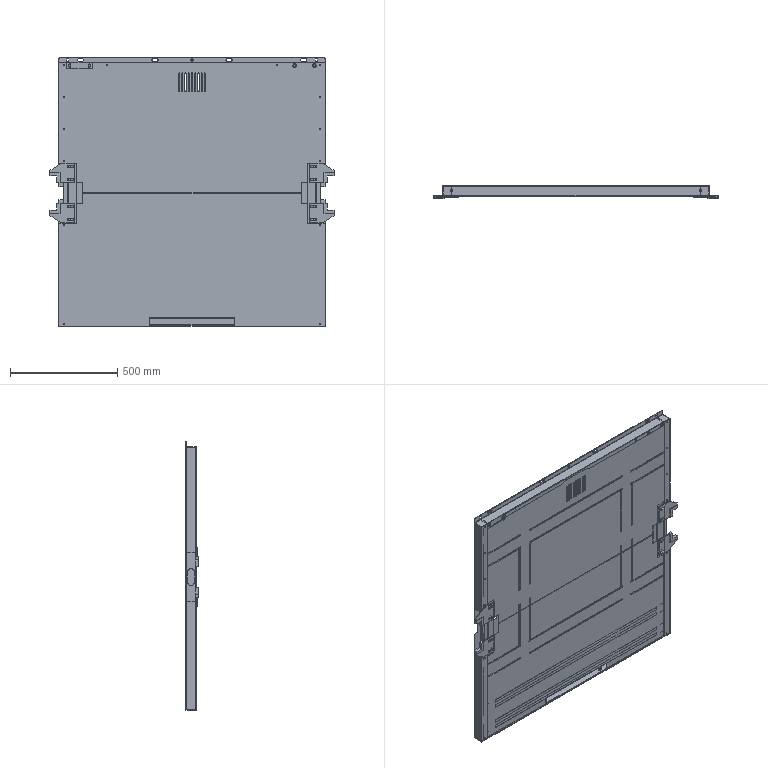Part | 27 solids | 1558 faces | box 1324 x 59.5 x 1250 mm | volume 6348848 mm3 | plane 1112 | cylinder 422 | cone 24 | commonest cylinder face diameters 10 x84 0.4 x70 11 x53 3.4 x44 5 x28 20 x27